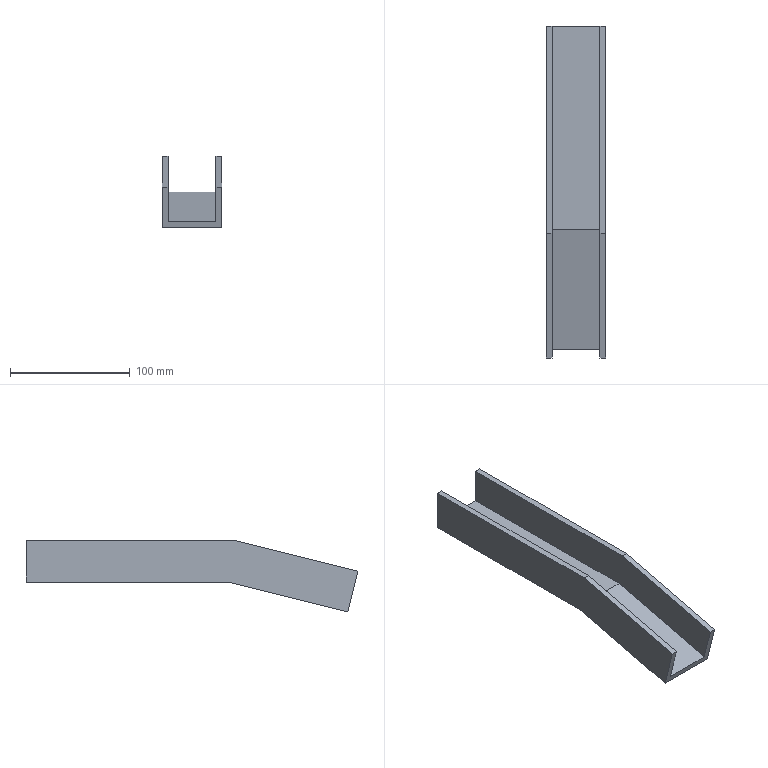Part | NX | features solid 2 | 1 solid | 14 faces | box 50 x 277.417 x 59.776 mm | volume 151230 mm3 | plane 14
STEP:
#1=CARTESIAN_POINT('',(-302.258,-1148.,-20.));
#2=VERTEX_POINT('',#1);
#3=CARTESIAN_POINT('',(-302.258,-1317.,-20.));
#4=VERTEX_POINT('',#3);
#5=CARTESIAN_POINT('',(-302.258,-1272.5,-20.));
#6=DIRECTION('',(0.,-1.,0.));
#7=VECTOR('',#6,1000.);
#8=LINE('',#5,#7);
#9=EDGE_CURVE('',#2,#4,#8,.T.);
#10=ORIENTED_EDGE('',*,*,#9,.F.);
#11=CARTESIAN_POINT('',(-252.258,-1148.,-20.));
#12=VERTEX_POINT('',#11);
#13=CARTESIAN_POINT('',(-252.258,-1148.,-20.));
#14=DIRECTION('',(1.,0.,0.));
#15=VECTOR('',#14,1000.);
#16=LINE('',#13,#15);
#17=EDGE_CURVE('',#2,#12,#16,.T.);
#18=ORIENTED_EDGE('',*,*,#17,.T.);
#19=CARTESIAN_POINT('',(-252.258,-1317.,-20.));
#20=VERTEX_POINT('',#19);
#21=CARTESIAN_POINT('',(-252.258,-1272.5,-20.));
#22=DIRECTION('',(0.,-1.,0.));
#23=VECTOR('',#22,1000.);
#24=LINE('',#21,#23);
#25=EDGE_CURVE('',#12,#20,#24,.T.);
#26=ORIENTED_EDGE('',*,*,#25,.T.);
#27=CARTESIAN_POINT('',(-277.258,-1317.,-20.));
#28=DIRECTION('',(1.,0.,0.));
#29=VECTOR('',#28,1000.);
#30=LINE('',#27,#29);
#31=EDGE_CURVE('',#4,#20,#30,.T.);
#32=ORIENTED_EDGE('',*,*,#31,.F.);
#33=EDGE_LOOP('',(#10,#18,#26,#32));
#34=FACE_BOUND('',#33,.T.);
#35=CARTESIAN_POINT('',(-252.258,-1272.5,-20.));
#36=DIRECTION('',(0.,0.,-1.));
#37=DIRECTION('',(0.,1.,0.));
#38=AXIS2_PLACEMENT_3D('',#35,#36,#37);
#39=PLANE('',#38);
#40=ADVANCED_FACE('',(#34),#39,.T.);
#41=CARTESIAN_POINT('',(-252.258,-1148.,15.));
#42=VERTEX_POINT('',#41);
#43=CARTESIAN_POINT('',(-257.258,-1148.,15.));
#44=VERTEX_POINT('',#43);
#45=CARTESIAN_POINT('',(-257.258,-1148.,15.));
#46=DIRECTION('',(-1.,0.,0.));
#47=VECTOR('',#46,1000.);
#48=LINE('',#45,#47);
#49=EDGE_CURVE('',#42,#44,#48,.T.);
#50=ORIENTED_EDGE('',*,*,#49,.F.);
#51=CARTESIAN_POINT('',(-252.258,-1148.,15.));
#52=DIRECTION('',(0.,0.,1.));
#53=VECTOR('',#52,1000.);
#54=LINE('',#51,#53);
#55=EDGE_CURVE('',#12,#42,#54,.T.);
#56=ORIENTED_EDGE('',*,*,#55,.F.);
#57=ORIENTED_EDGE('',*,*,#17,.F.);
#58=CARTESIAN_POINT('',(-302.258,-1148.,15.));
#59=VERTEX_POINT('',#58);
#60=CARTESIAN_POINT('',(-302.258,-1148.,15.));
#61=DIRECTION('',(0.,0.,-1.));
#62=VECTOR('',#61,1000.);
#63=LINE('',#60,#62);
#64=EDGE_CURVE('',#59,#2,#63,.T.);
#65=ORIENTED_EDGE('',*,*,#64,.F.);
#66=CARTESIAN_POINT('',(-297.258,-1148.,15.));
#67=VERTEX_POINT('',#66);
#68=CARTESIAN_POINT('',(-302.258,-1148.,15.));
#69=DIRECTION('',(-1.,0.,0.));
#70=VECTOR('',#69,1000.);
#71=LINE('',#68,#70);
#72=EDGE_CURVE('',#67,#59,#71,.T.);
#73=ORIENTED_EDGE('',*,*,#72,.F.);
#74=CARTESIAN_POINT('',(-297.258,-1148.,-15.));
#75=VERTEX_POINT('',#74);
#76=CARTESIAN_POINT('',(-297.258,-1148.,15.));
#77=DIRECTION('',(0.,0.,1.));
#78=VECTOR('',#77,1000.);
#79=LINE('',#76,#78);
#80=EDGE_CURVE('',#75,#67,#79,.T.);
#81=ORIENTED_EDGE('',*,*,#80,.F.);
#82=CARTESIAN_POINT('',(-257.258,-1148.,-15.));
#83=VERTEX_POINT('',#82);
#84=CARTESIAN_POINT('',(-297.258,-1148.,-15.));
#85=DIRECTION('',(-1.,0.,0.));
#86=VECTOR('',#85,1000.);
#87=LINE('',#84,#86);
#88=EDGE_CURVE('',#83,#75,#87,.T.);
#89=ORIENTED_EDGE('',*,*,#88,.F.);
#90=CARTESIAN_POINT('',(-257.258,-1148.,15.));
#91=DIRECTION('',(0.,0.,-1.));
#92=VECTOR('',#91,1000.);
#93=LINE('',#90,#92);
#94=EDGE_CURVE('',#44,#83,#93,.T.);
#95=ORIENTED_EDGE('',*,*,#94,.F.);
#96=EDGE_LOOP('',(#50,#56,#57,#65,#73,#81,#89,#95));
#97=FACE_BOUND('',#96,.T.);
#98=CARTESIAN_POINT('',(-252.258,-1148.,15.));
#99=DIRECTION('',(0.,1.,0.));
#100=DIRECTION('',(0.,0.,1.));
#101=AXIS2_PLACEMENT_3D('',#98,#99,#100);
#102=PLANE('',#101);
#103=ADVANCED_FACE('',(#97),#102,.T.);
#104=CARTESIAN_POINT('',(-297.258,-1418.202,-39.923));
#105=VERTEX_POINT('',#104);
#106=CARTESIAN_POINT('',(-297.258,-1425.417,-10.804));
#107=VERTEX_POINT('',#106);
#108=CARTESIAN_POINT('',(-297.258,-1421.81,-25.363));
#109=DIRECTION('',(0.,-0.2405,0.9707));
#110=VECTOR('',#109,1000.);
#111=LINE('',#108,#110);
#112=EDGE_CURVE('',#105,#107,#111,.T.);
#113=ORIENTED_EDGE('',*,*,#112,.T.);
#114=CARTESIAN_POINT('',(-302.258,-1425.417,-10.804));
#115=VERTEX_POINT('',#114);
#116=CARTESIAN_POINT('',(-299.758,-1425.417,-10.804));
#117=DIRECTION('',(-1.,0.,0.));
#118=VECTOR('',#117,1000.);
#119=LINE('',#116,#118);
#120=EDGE_CURVE('',#107,#115,#119,.T.);
#121=ORIENTED_EDGE('',*,*,#120,.T.);
#122=CARTESIAN_POINT('',(-302.258,-1417.,-44.776));
#123=VERTEX_POINT('',#122);
#124=CARTESIAN_POINT('',(-302.258,-1421.209,-27.79));
#125=DIRECTION('',(0.,0.2405,-0.9707));
#126=VECTOR('',#125,1000.);
#127=LINE('',#124,#126);
#128=EDGE_CURVE('',#115,#123,#127,.T.);
#129=ORIENTED_EDGE('',*,*,#128,.T.);
#130=CARTESIAN_POINT('',(-252.258,-1417.,-44.776));
#131=VERTEX_POINT('',#130);
#132=CARTESIAN_POINT('',(-277.258,-1417.,-44.776));
#133=DIRECTION('',(1.,0.,0.));
#134=VECTOR('',#133,1000.);
#135=LINE('',#132,#134);
#136=EDGE_CURVE('',#123,#131,#135,.T.);
#137=ORIENTED_EDGE('',*,*,#136,.T.);
#138=CARTESIAN_POINT('',(-252.258,-1425.417,-10.804));
#139=VERTEX_POINT('',#138);
#140=CARTESIAN_POINT('',(-252.258,-1421.209,-27.79));
#141=DIRECTION('',(0.,-0.2405,0.9707));
#142=VECTOR('',#141,1000.);
#143=LINE('',#140,#142);
#144=EDGE_CURVE('',#131,#139,#143,.T.);
#145=ORIENTED_EDGE('',*,*,#144,.T.);
#146=CARTESIAN_POINT('',(-257.258,-1425.417,-10.804));
#147=VERTEX_POINT('',#146);
#148=CARTESIAN_POINT('',(-254.758,-1425.417,-10.804));
#149=DIRECTION('',(-1.,0.,0.));
#150=VECTOR('',#149,1000.);
#151=LINE('',#148,#150);
#152=EDGE_CURVE('',#139,#147,#151,.T.);
#153=ORIENTED_EDGE('',*,*,#152,.T.);
#154=CARTESIAN_POINT('',(-257.258,-1418.202,-39.923));
#155=VERTEX_POINT('',#154);
#156=CARTESIAN_POINT('',(-257.258,-1421.81,-25.363));
#157=DIRECTION('',(0.,0.2405,-0.9707));
#158=VECTOR('',#157,1000.);
#159=LINE('',#156,#158);
#160=EDGE_CURVE('',#147,#155,#159,.T.);
#161=ORIENTED_EDGE('',*,*,#160,.T.);
#162=CARTESIAN_POINT('',(-277.258,-1418.202,-39.923));
#163=DIRECTION('',(-1.,0.,0.));
#164=VECTOR('',#163,1000.);
#165=LINE('',#162,#164);
#166=EDGE_CURVE('',#155,#105,#165,.T.);
#167=ORIENTED_EDGE('',*,*,#166,.T.);
#168=EDGE_LOOP('',(#113,#121,#129,#137,#145,#153,#161,#167));
#169=FACE_BOUND('',#168,.T.);
#170=CARTESIAN_POINT('',(-277.258,-1417.,-44.776));
#171=DIRECTION('',(0.,-0.9707,-0.2405));
#172=DIRECTION('',(0.,0.2405,-0.9707));
#173=AXIS2_PLACEMENT_3D('',#170,#171,#172);
#174=PLANE('',#173);
#175=ADVANCED_FACE('',(#169),#174,.T.);
#176=CARTESIAN_POINT('',(-297.258,-1321.271,15.));
#177=VERTEX_POINT('',#176);
#178=CARTESIAN_POINT('',(-297.258,-1373.344,2.098));
#179=DIRECTION('',(0.,-0.9707,-0.2405));
#180=VECTOR('',#179,1000.);
#181=LINE('',#178,#180);
#182=EDGE_CURVE('',#177,#107,#181,.T.);
#183=ORIENTED_EDGE('',*,*,#182,.F.);
#184=CARTESIAN_POINT('',(-302.258,-1321.271,15.));
#185=VERTEX_POINT('',#184);
#186=CARTESIAN_POINT('',(-299.758,-1321.271,15.));
#187=DIRECTION('',(-1.,0.,0.));
#188=VECTOR('',#187,1000.);
#189=LINE('',#186,#188);
#190=EDGE_CURVE('',#177,#185,#189,.T.);
#191=ORIENTED_EDGE('',*,*,#190,.T.);
#192=CARTESIAN_POINT('',(-302.258,-1373.344,2.098));
#193=DIRECTION('',(0.,-0.9707,-0.2405));
#194=VECTOR('',#193,1000.);
#195=LINE('',#192,#194);
#196=EDGE_CURVE('',#185,#115,#195,.T.);
#197=ORIENTED_EDGE('',*,*,#196,.T.);
#198=ORIENTED_EDGE('',*,*,#120,.F.);
#199=EDGE_LOOP('',(#183,#191,#197,#198));
#200=FACE_BOUND('',#199,.T.);
#201=CARTESIAN_POINT('',(-302.258,-1373.344,2.098));
#202=DIRECTION('',(0.,-0.2405,0.9707));
#203=DIRECTION('',(0.,-0.9707,-0.2405));
#204=AXIS2_PLACEMENT_3D('',#201,#202,#203);
#205=PLANE('',#204);
#206=ADVANCED_FACE('',(#200),#205,.T.);
#207=CARTESIAN_POINT('',(-297.258,-1317.61,-15.));
#208=VERTEX_POINT('',#207);
#209=CARTESIAN_POINT('',(-297.258,-1272.805,-15.));
#210=DIRECTION('',(0.,-1.,0.));
#211=VECTOR('',#210,1000.);
#212=LINE('',#209,#211);
#213=EDGE_CURVE('',#75,#208,#212,.T.);
#214=ORIENTED_EDGE('',*,*,#213,.F.);
#215=ORIENTED_EDGE('',*,*,#80,.T.);
#216=CARTESIAN_POINT('',(-297.258,-1274.636,15.));
#217=DIRECTION('',(0.,-1.,0.));
#218=VECTOR('',#217,1000.);
#219=LINE('',#216,#218);
#220=EDGE_CURVE('',#67,#177,#219,.T.);
#221=ORIENTED_EDGE('',*,*,#220,.T.);
#222=ORIENTED_EDGE('',*,*,#182,.T.);
#223=ORIENTED_EDGE('',*,*,#112,.F.);
#224=CARTESIAN_POINT('',(-297.258,-1367.906,-27.462));
#225=DIRECTION('',(0.,-0.9707,-0.2405));
#226=VECTOR('',#225,1000.);
#227=LINE('',#224,#226);
#228=EDGE_CURVE('',#208,#105,#227,.T.);
#229=ORIENTED_EDGE('',*,*,#228,.F.);
#230=EDGE_LOOP('',(#214,#215,#221,#222,#223,#229));
#231=FACE_BOUND('',#230,.T.);
#232=CARTESIAN_POINT('',(-297.258,-1274.636,15.));
#233=DIRECTION('',(1.,0.,0.));
#234=DIRECTION('',(0.,0.,1.));
#235=AXIS2_PLACEMENT_3D('',#232,#233,#234);
#236=PLANE('',#235);
#237=ADVANCED_FACE('',(#231),#236,.T.);
#238=CARTESIAN_POINT('',(-257.258,-1317.61,-15.));
#239=VERTEX_POINT('',#238);
#240=CARTESIAN_POINT('',(-257.258,-1367.906,-27.462));
#241=DIRECTION('',(0.,-0.9707,-0.2405));
#242=VECTOR('',#241,1000.);
#243=LINE('',#240,#242);
#244=EDGE_CURVE('',#239,#155,#243,.T.);
#245=ORIENTED_EDGE('',*,*,#244,.F.);
#246=CARTESIAN_POINT('',(-277.258,-1317.61,-15.));
#247=DIRECTION('',(-1.,0.,0.));
#248=VECTOR('',#247,1000.);
#249=LINE('',#246,#248);
#250=EDGE_CURVE('',#239,#208,#249,.T.);
#251=ORIENTED_EDGE('',*,*,#250,.T.);
#252=ORIENTED_EDGE('',*,*,#228,.T.);
#253=ORIENTED_EDGE('',*,*,#166,.F.);
#254=EDGE_LOOP('',(#245,#251,#252,#253));
#255=FACE_BOUND('',#254,.T.);
#256=CARTESIAN_POINT('',(-297.258,-1367.906,-27.462));
#257=DIRECTION('',(0.,-0.2405,0.9707));
#258=DIRECTION('',(0.,-0.9707,-0.2405));
#259=AXIS2_PLACEMENT_3D('',#256,#257,#258);
#260=PLANE('',#259);
#261=ADVANCED_FACE('',(#255),#260,.T.);
#262=CARTESIAN_POINT('',(-257.258,-1272.805,-15.));
#263=DIRECTION('',(0.,-1.,0.));
#264=VECTOR('',#263,1000.);
#265=LINE('',#262,#264);
#266=EDGE_CURVE('',#83,#239,#265,.T.);
#267=ORIENTED_EDGE('',*,*,#266,.F.);
#268=ORIENTED_EDGE('',*,*,#88,.T.);
#269=ORIENTED_EDGE('',*,*,#213,.T.);
#270=ORIENTED_EDGE('',*,*,#250,.F.);
#271=EDGE_LOOP('',(#267,#268,#269,#270));
#272=FACE_BOUND('',#271,.T.);
#273=CARTESIAN_POINT('',(-297.258,-1272.805,-15.));
#274=DIRECTION('',(0.,0.,1.));
#275=DIRECTION('',(0.,-1.,0.));
#276=AXIS2_PLACEMENT_3D('',#273,#274,#275);
#277=PLANE('',#276);
#278=ADVANCED_FACE('',(#272),#277,.T.);
#279=CARTESIAN_POINT('',(-257.258,-1321.271,15.));
#280=VERTEX_POINT('',#279);
#281=CARTESIAN_POINT('',(-257.258,-1274.636,15.));
#282=DIRECTION('',(0.,-1.,0.));
#283=VECTOR('',#282,1000.);
#284=LINE('',#281,#283);
#285=EDGE_CURVE('',#44,#280,#284,.T.);
#286=ORIENTED_EDGE('',*,*,#285,.F.);
#287=ORIENTED_EDGE('',*,*,#94,.T.);
#288=ORIENTED_EDGE('',*,*,#266,.T.);
#289=ORIENTED_EDGE('',*,*,#244,.T.);
#290=ORIENTED_EDGE('',*,*,#160,.F.);
#291=CARTESIAN_POINT('',(-257.258,-1373.344,2.098));
#292=DIRECTION('',(0.,-0.9707,-0.2405));
#293=VECTOR('',#292,1000.);
#294=LINE('',#291,#293);
#295=EDGE_CURVE('',#280,#147,#294,.T.);
#296=ORIENTED_EDGE('',*,*,#295,.F.);
#297=EDGE_LOOP('',(#286,#287,#288,#289,#290,#296));
#298=FACE_BOUND('',#297,.T.);
#299=CARTESIAN_POINT('',(-257.258,-1274.636,15.));
#300=DIRECTION('',(-1.,0.,0.));
#301=DIRECTION('',(0.,0.,-1.));
#302=AXIS2_PLACEMENT_3D('',#299,#300,#301);
#303=PLANE('',#302);
#304=ADVANCED_FACE('',(#298),#303,.T.);
#305=CARTESIAN_POINT('',(-252.258,-1321.271,15.));
#306=VERTEX_POINT('',#305);
#307=CARTESIAN_POINT('',(-252.258,-1373.344,2.098));
#308=DIRECTION('',(0.,-0.9707,-0.2405));
#309=VECTOR('',#308,1000.);
#310=LINE('',#307,#309);
#311=EDGE_CURVE('',#306,#139,#310,.T.);
#312=ORIENTED_EDGE('',*,*,#311,.F.);
#313=CARTESIAN_POINT('',(-254.758,-1321.271,15.));
#314=DIRECTION('',(-1.,0.,0.));
#315=VECTOR('',#314,1000.);
#316=LINE('',#313,#315);
#317=EDGE_CURVE('',#306,#280,#316,.T.);
#318=ORIENTED_EDGE('',*,*,#317,.T.);
#319=ORIENTED_EDGE('',*,*,#295,.T.);
#320=ORIENTED_EDGE('',*,*,#152,.F.);
#321=EDGE_LOOP('',(#312,#318,#319,#320));
#322=FACE_BOUND('',#321,.T.);
#323=CARTESIAN_POINT('',(-257.258,-1373.344,2.098));
#324=DIRECTION('',(0.,-0.2405,0.9707));
#325=DIRECTION('',(0.,-0.9707,-0.2405));
#326=AXIS2_PLACEMENT_3D('',#323,#324,#325);
#327=PLANE('',#326);
#328=ADVANCED_FACE('',(#322),#327,.T.);
#329=CARTESIAN_POINT('',(-252.258,-1274.636,15.));
#330=DIRECTION('',(0.,-1.,0.));
#331=VECTOR('',#330,1000.);
#332=LINE('',#329,#331);
#333=EDGE_CURVE('',#42,#306,#332,.T.);
#334=ORIENTED_EDGE('',*,*,#333,.F.);
#335=ORIENTED_EDGE('',*,*,#49,.T.);
#336=ORIENTED_EDGE('',*,*,#285,.T.);
#337=ORIENTED_EDGE('',*,*,#317,.F.);
#338=EDGE_LOOP('',(#334,#335,#336,#337));
#339=FACE_BOUND('',#338,.T.);
#340=CARTESIAN_POINT('',(-257.258,-1274.636,15.));
#341=DIRECTION('',(0.,0.,1.));
#342=DIRECTION('',(0.,-1.,0.));
#343=AXIS2_PLACEMENT_3D('',#340,#341,#342);
#344=PLANE('',#343);
#345=ADVANCED_FACE('',(#339),#344,.T.);
#346=ORIENTED_EDGE('',*,*,#25,.F.);
#347=ORIENTED_EDGE('',*,*,#55,.T.);
#348=ORIENTED_EDGE('',*,*,#333,.T.);
#349=ORIENTED_EDGE('',*,*,#311,.T.);
#350=ORIENTED_EDGE('',*,*,#144,.F.);
#351=CARTESIAN_POINT('',(-252.258,-1367.,-32.388));
#352=DIRECTION('',(0.,-0.9707,-0.2405));
#353=VECTOR('',#352,1000.);
#354=LINE('',#351,#353);
#355=EDGE_CURVE('',#20,#131,#354,.T.);
#356=ORIENTED_EDGE('',*,*,#355,.F.);
#357=EDGE_LOOP('',(#346,#347,#348,#349,#350,#356));
#358=FACE_BOUND('',#357,.T.);
#359=CARTESIAN_POINT('',(-252.258,-1274.636,15.));
#360=DIRECTION('',(1.,0.,0.));
#361=DIRECTION('',(0.,0.,1.));
#362=AXIS2_PLACEMENT_3D('',#359,#360,#361);
#363=PLANE('',#362);
#364=ADVANCED_FACE('',(#358),#363,.T.);
#365=CARTESIAN_POINT('',(-302.258,-1367.,-32.388));
#366=DIRECTION('',(0.,-0.9707,-0.2405));
#367=VECTOR('',#366,1000.);
#368=LINE('',#365,#367);
#369=EDGE_CURVE('',#4,#123,#368,.T.);
#370=ORIENTED_EDGE('',*,*,#369,.F.);
#371=ORIENTED_EDGE('',*,*,#31,.T.);
#372=ORIENTED_EDGE('',*,*,#355,.T.);
#373=ORIENTED_EDGE('',*,*,#136,.F.);
#374=EDGE_LOOP('',(#370,#371,#372,#373));
#375=FACE_BOUND('',#374,.T.);
#376=CARTESIAN_POINT('',(-252.258,-1367.,-32.388));
#377=DIRECTION('',(0.,0.2405,-0.9707));
#378=DIRECTION('',(0.,0.9707,0.2405));
#379=AXIS2_PLACEMENT_3D('',#376,#377,#378);
#380=PLANE('',#379);
#381=ADVANCED_FACE('',(#375),#380,.T.);
#382=ORIENTED_EDGE('',*,*,#220,.F.);
#383=ORIENTED_EDGE('',*,*,#72,.T.);
#384=CARTESIAN_POINT('',(-302.258,-1274.636,15.));
#385=DIRECTION('',(0.,-1.,0.));
#386=VECTOR('',#385,1000.);
#387=LINE('',#384,#386);
#388=EDGE_CURVE('',#59,#185,#387,.T.);
#389=ORIENTED_EDGE('',*,*,#388,.T.);
#390=ORIENTED_EDGE('',*,*,#190,.F.);
#391=EDGE_LOOP('',(#382,#383,#389,#390));
#392=FACE_BOUND('',#391,.T.);
#393=CARTESIAN_POINT('',(-302.258,-1274.636,15.));
#394=DIRECTION('',(0.,0.,1.));
#395=DIRECTION('',(0.,-1.,0.));
#396=AXIS2_PLACEMENT_3D('',#393,#394,#395);
#397=PLANE('',#396);
#398=ADVANCED_FACE('',(#392),#397,.T.);
#399=ORIENTED_EDGE('',*,*,#388,.F.);
#400=ORIENTED_EDGE('',*,*,#64,.T.);
#401=ORIENTED_EDGE('',*,*,#9,.T.);
#402=ORIENTED_EDGE('',*,*,#369,.T.);
#403=ORIENTED_EDGE('',*,*,#128,.F.);
#404=ORIENTED_EDGE('',*,*,#196,.F.);
#405=EDGE_LOOP('',(#399,#400,#401,#402,#403,#404));
#406=FACE_BOUND('',#405,.T.);
#407=CARTESIAN_POINT('',(-302.258,-1274.636,15.));
#408=DIRECTION('',(-1.,0.,0.));
#409=DIRECTION('',(0.,0.,-1.));
#410=AXIS2_PLACEMENT_3D('',#407,#408,#409);
#411=PLANE('',#410);
#412=ADVANCED_FACE('',(#406),#411,.T.);
#413=CLOSED_SHELL('',(#40,#103,#175,#206,#237,#261,#278,#304,#328,#345,#364,#381,#398,#412));
#414=MANIFOLD_SOLID_BREP('',#413);
#415=(LENGTH_UNIT()NAMED_UNIT(*)SI_UNIT(.MILLI.,.METRE.));
#416=UNCERTAINTY_MEASURE_WITH_UNIT(LENGTH_MEASURE(0.00001),#415,'','');
#417=(NAMED_UNIT(*)PLANE_ANGLE_UNIT()SI_UNIT($,.RADIAN.));
#418=(NAMED_UNIT(*)SI_UNIT($,.STERADIAN.)SOLID_ANGLE_UNIT());
#419=(GEOMETRIC_REPRESENTATION_CONTEXT(3)GLOBAL_UNCERTAINTY_ASSIGNED_CONTEXT((#416))GLOBAL_UNIT_ASSIGNED_CONTEXT((#415,#417,#418))REPRESENTATION_CONTEXT('',''));
#420=ADVANCED_BREP_SHAPE_REPRESENTATION('',(#414),#419);